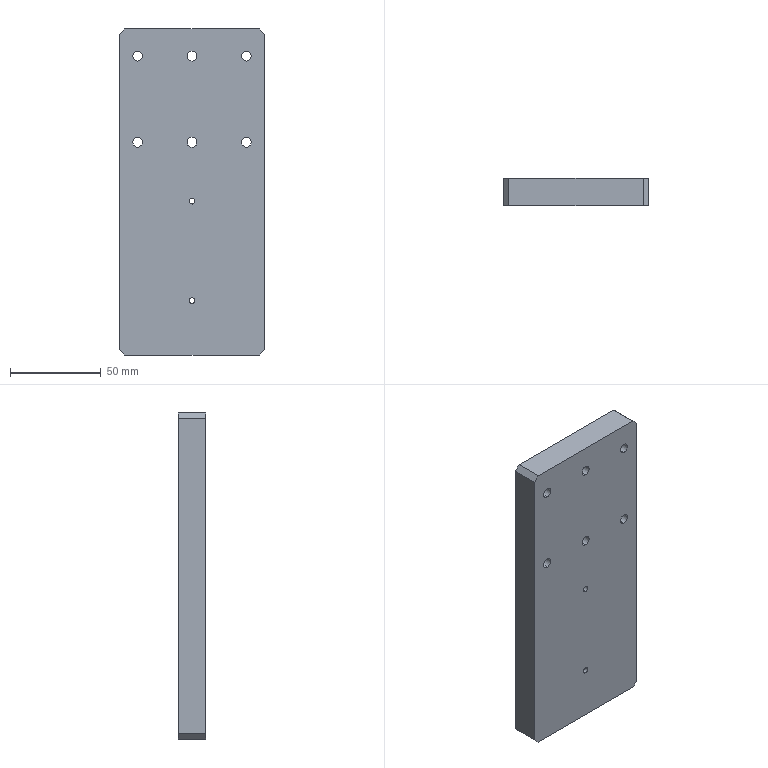Part | SolidWorks | features HoleWzd 3, Chamfer 1, Extrusion 1 | 1 solid | 44 faces | box 80 x 15 x 180 mm | volume 211462 mm3 | cylinder 28 | plane 16 | commonest cylinder face diameters 5.5 x12 10 x12 3.3 x4
STEP:
#1=CARTESIAN_POINT('',(-30.,9.3,70.));
#2=VERTEX_POINT('',#1);
#3=CARTESIAN_POINT('',(-30.,9.3,80.));
#4=VERTEX_POINT('',#3);
#5=CARTESIAN_POINT('',(-30.,9.3,75.));
#6=DIRECTION('',(0.,1.,0.));
#7=DIRECTION('',(0.,0.,1.));
#8=AXIS2_PLACEMENT_3D('',#5,#6,#7);
#9=CIRCLE('',#8,5.);
#10=EDGE_CURVE('',#2,#4,#9,.T.);
#11=ORIENTED_EDGE('',*,*,#10,.F.);
#12=CARTESIAN_POINT('',(-30.,15.,70.));
#13=VERTEX_POINT('',#12);
#14=CARTESIAN_POINT('',(-30.,15.,70.));
#15=DIRECTION('',(0.,1.,0.));
#16=VECTOR('',#15,1000.);
#17=LINE('',#14,#16);
#18=EDGE_CURVE('',#2,#13,#17,.T.);
#19=ORIENTED_EDGE('',*,*,#18,.T.);
#20=CARTESIAN_POINT('',(-30.,15.,80.));
#21=VERTEX_POINT('',#20);
#22=CARTESIAN_POINT('',(-30.,15.,75.));
#23=DIRECTION('',(0.,1.,0.));
#24=DIRECTION('',(0.,0.,1.));
#25=AXIS2_PLACEMENT_3D('',#22,#23,#24);
#26=CIRCLE('',#25,5.);
#27=EDGE_CURVE('',#13,#21,#26,.T.);
#28=ORIENTED_EDGE('',*,*,#27,.T.);
#29=CARTESIAN_POINT('',(-30.,15.,80.));
#30=DIRECTION('',(0.,1.,0.));
#31=VECTOR('',#30,1000.);
#32=LINE('',#29,#31);
#33=EDGE_CURVE('',#4,#21,#32,.T.);
#34=ORIENTED_EDGE('',*,*,#33,.F.);
#35=EDGE_LOOP('',(#11,#19,#28,#34));
#36=FACE_OUTER_BOUND('',#35,.T.);
#37=CARTESIAN_POINT('',(-30.,15.,75.));
#38=DIRECTION('',(0.,1.,0.));
#39=DIRECTION('',(0.,0.,1.));
#40=AXIS2_PLACEMENT_3D('',#37,#38,#39);
#41=CYLINDRICAL_SURFACE('',#40,5.);
#42=ADVANCED_FACE('',(#36),#41,.F.);
#43=CARTESIAN_POINT('',(-30.,0.,72.25));
#44=VERTEX_POINT('',#43);
#45=CARTESIAN_POINT('',(-30.,0.,77.75));
#46=VERTEX_POINT('',#45);
#47=CARTESIAN_POINT('',(-30.,0.,75.));
#48=DIRECTION('',(0.,1.,0.));
#49=DIRECTION('',(0.,0.,1.));
#50=AXIS2_PLACEMENT_3D('',#47,#48,#49);
#51=CIRCLE('',#50,2.75);
#52=EDGE_CURVE('',#44,#46,#51,.T.);
#53=ORIENTED_EDGE('',*,*,#52,.F.);
#54=CARTESIAN_POINT('',(-30.,9.3,72.25));
#55=VERTEX_POINT('',#54);
#56=CARTESIAN_POINT('',(-30.,15.,72.25));
#57=DIRECTION('',(0.,1.,0.));
#58=VECTOR('',#57,1000.);
#59=LINE('',#56,#58);
#60=EDGE_CURVE('',#44,#55,#59,.T.);
#61=ORIENTED_EDGE('',*,*,#60,.T.);
#62=CARTESIAN_POINT('',(-30.,9.3,77.75));
#63=VERTEX_POINT('',#62);
#64=CARTESIAN_POINT('',(-30.,9.3,75.));
#65=DIRECTION('',(0.,1.,0.));
#66=DIRECTION('',(0.,0.,1.));
#67=AXIS2_PLACEMENT_3D('',#64,#65,#66);
#68=CIRCLE('',#67,2.75);
#69=EDGE_CURVE('',#55,#63,#68,.T.);
#70=ORIENTED_EDGE('',*,*,#69,.T.);
#71=CARTESIAN_POINT('',(-30.,15.,77.75));
#72=DIRECTION('',(0.,1.,0.));
#73=VECTOR('',#72,1000.);
#74=LINE('',#71,#73);
#75=EDGE_CURVE('',#46,#63,#74,.T.);
#76=ORIENTED_EDGE('',*,*,#75,.F.);
#77=EDGE_LOOP('',(#53,#61,#70,#76));
#78=FACE_OUTER_BOUND('',#77,.T.);
#79=CARTESIAN_POINT('',(-30.,15.,75.));
#80=DIRECTION('',(0.,1.,0.));
#81=DIRECTION('',(0.,0.,1.));
#82=AXIS2_PLACEMENT_3D('',#79,#80,#81);
#83=CYLINDRICAL_SURFACE('',#82,2.75);
#84=ADVANCED_FACE('',(#78),#83,.F.);
#85=CARTESIAN_POINT('',(0.,9.3,70.));
#86=VERTEX_POINT('',#85);
#87=CARTESIAN_POINT('',(0.,9.3,80.));
#88=VERTEX_POINT('',#87);
#89=CARTESIAN_POINT('',(0.,9.3,75.));
#90=DIRECTION('',(0.,1.,0.));
#91=DIRECTION('',(0.,0.,1.));
#92=AXIS2_PLACEMENT_3D('',#89,#90,#91);
#93=CIRCLE('',#92,5.);
#94=EDGE_CURVE('',#86,#88,#93,.T.);
#95=ORIENTED_EDGE('',*,*,#94,.F.);
#96=CARTESIAN_POINT('',(0.,15.,70.));
#97=VERTEX_POINT('',#96);
#98=CARTESIAN_POINT('',(0.,15.,70.));
#99=DIRECTION('',(0.,1.,0.));
#100=VECTOR('',#99,1000.);
#101=LINE('',#98,#100);
#102=EDGE_CURVE('',#86,#97,#101,.T.);
#103=ORIENTED_EDGE('',*,*,#102,.T.);
#104=CARTESIAN_POINT('',(0.,15.,80.));
#105=VERTEX_POINT('',#104);
#106=CARTESIAN_POINT('',(0.,15.,75.));
#107=DIRECTION('',(0.,1.,0.));
#108=DIRECTION('',(0.,0.,1.));
#109=AXIS2_PLACEMENT_3D('',#106,#107,#108);
#110=CIRCLE('',#109,5.);
#111=EDGE_CURVE('',#97,#105,#110,.T.);
#112=ORIENTED_EDGE('',*,*,#111,.T.);
#113=CARTESIAN_POINT('',(0.,15.,80.));
#114=DIRECTION('',(0.,1.,0.));
#115=VECTOR('',#114,1000.);
#116=LINE('',#113,#115);
#117=EDGE_CURVE('',#88,#105,#116,.T.);
#118=ORIENTED_EDGE('',*,*,#117,.F.);
#119=EDGE_LOOP('',(#95,#103,#112,#118));
#120=FACE_OUTER_BOUND('',#119,.T.);
#121=CARTESIAN_POINT('',(0.,15.,75.));
#122=DIRECTION('',(0.,1.,0.));
#123=DIRECTION('',(0.,0.,1.));
#124=AXIS2_PLACEMENT_3D('',#121,#122,#123);
#125=CYLINDRICAL_SURFACE('',#124,5.);
#126=ADVANCED_FACE('',(#120),#125,.F.);
#127=CARTESIAN_POINT('',(0.,0.,72.25));
#128=VERTEX_POINT('',#127);
#129=CARTESIAN_POINT('',(0.,0.,77.75));
#130=VERTEX_POINT('',#129);
#131=CARTESIAN_POINT('',(0.,0.,75.));
#132=DIRECTION('',(0.,1.,0.));
#133=DIRECTION('',(0.,0.,1.));
#134=AXIS2_PLACEMENT_3D('',#131,#132,#133);
#135=CIRCLE('',#134,2.75);
#136=EDGE_CURVE('',#128,#130,#135,.T.);
#137=ORIENTED_EDGE('',*,*,#136,.F.);
#138=CARTESIAN_POINT('',(0.,9.3,72.25));
#139=VERTEX_POINT('',#138);
#140=CARTESIAN_POINT('',(0.,15.,72.25));
#141=DIRECTION('',(0.,1.,0.));
#142=VECTOR('',#141,1000.);
#143=LINE('',#140,#142);
#144=EDGE_CURVE('',#128,#139,#143,.T.);
#145=ORIENTED_EDGE('',*,*,#144,.T.);
#146=CARTESIAN_POINT('',(0.,9.3,77.75));
#147=VERTEX_POINT('',#146);
#148=CARTESIAN_POINT('',(0.,9.3,75.));
#149=DIRECTION('',(0.,1.,0.));
#150=DIRECTION('',(0.,0.,1.));
#151=AXIS2_PLACEMENT_3D('',#148,#149,#150);
#152=CIRCLE('',#151,2.75);
#153=EDGE_CURVE('',#139,#147,#152,.T.);
#154=ORIENTED_EDGE('',*,*,#153,.T.);
#155=CARTESIAN_POINT('',(0.,15.,77.75));
#156=DIRECTION('',(0.,1.,0.));
#157=VECTOR('',#156,1000.);
#158=LINE('',#155,#157);
#159=EDGE_CURVE('',#130,#147,#158,.T.);
#160=ORIENTED_EDGE('',*,*,#159,.F.);
#161=EDGE_LOOP('',(#137,#145,#154,#160));
#162=FACE_OUTER_BOUND('',#161,.T.);
#163=CARTESIAN_POINT('',(0.,15.,75.));
#164=DIRECTION('',(0.,1.,0.));
#165=DIRECTION('',(0.,0.,1.));
#166=AXIS2_PLACEMENT_3D('',#163,#164,#165);
#167=CYLINDRICAL_SURFACE('',#166,2.75);
#168=ADVANCED_FACE('',(#162),#167,.F.);
#169=CARTESIAN_POINT('',(30.,9.3,70.));
#170=VERTEX_POINT('',#169);
#171=CARTESIAN_POINT('',(30.,9.3,80.));
#172=VERTEX_POINT('',#171);
#173=CARTESIAN_POINT('',(30.,9.3,75.));
#174=DIRECTION('',(0.,1.,0.));
#175=DIRECTION('',(0.,0.,1.));
#176=AXIS2_PLACEMENT_3D('',#173,#174,#175);
#177=CIRCLE('',#176,5.);
#178=EDGE_CURVE('',#170,#172,#177,.T.);
#179=ORIENTED_EDGE('',*,*,#178,.F.);
#180=CARTESIAN_POINT('',(30.,15.,70.));
#181=VERTEX_POINT('',#180);
#182=CARTESIAN_POINT('',(30.,15.,70.));
#183=DIRECTION('',(0.,1.,0.));
#184=VECTOR('',#183,1000.);
#185=LINE('',#182,#184);
#186=EDGE_CURVE('',#170,#181,#185,.T.);
#187=ORIENTED_EDGE('',*,*,#186,.T.);
#188=CARTESIAN_POINT('',(30.,15.,80.));
#189=VERTEX_POINT('',#188);
#190=CARTESIAN_POINT('',(30.,15.,75.));
#191=DIRECTION('',(0.,1.,0.));
#192=DIRECTION('',(0.,0.,1.));
#193=AXIS2_PLACEMENT_3D('',#190,#191,#192);
#194=CIRCLE('',#193,5.);
#195=EDGE_CURVE('',#181,#189,#194,.T.);
#196=ORIENTED_EDGE('',*,*,#195,.T.);
#197=CARTESIAN_POINT('',(30.,15.,80.));
#198=DIRECTION('',(0.,1.,0.));
#199=VECTOR('',#198,1000.);
#200=LINE('',#197,#199);
#201=EDGE_CURVE('',#172,#189,#200,.T.);
#202=ORIENTED_EDGE('',*,*,#201,.F.);
#203=EDGE_LOOP('',(#179,#187,#196,#202));
#204=FACE_OUTER_BOUND('',#203,.T.);
#205=CARTESIAN_POINT('',(30.,15.,75.));
#206=DIRECTION('',(0.,1.,0.));
#207=DIRECTION('',(0.,0.,1.));
#208=AXIS2_PLACEMENT_3D('',#205,#206,#207);
#209=CYLINDRICAL_SURFACE('',#208,5.);
#210=ADVANCED_FACE('',(#204),#209,.F.);
#211=CARTESIAN_POINT('',(30.,0.,72.25));
#212=VERTEX_POINT('',#211);
#213=CARTESIAN_POINT('',(30.,0.,77.75));
#214=VERTEX_POINT('',#213);
#215=CARTESIAN_POINT('',(30.,0.,75.));
#216=DIRECTION('',(0.,1.,0.));
#217=DIRECTION('',(0.,0.,1.));
#218=AXIS2_PLACEMENT_3D('',#215,#216,#217);
#219=CIRCLE('',#218,2.75);
#220=EDGE_CURVE('',#212,#214,#219,.T.);
#221=ORIENTED_EDGE('',*,*,#220,.F.);
#222=CARTESIAN_POINT('',(30.,9.3,72.25));
#223=VERTEX_POINT('',#222);
#224=CARTESIAN_POINT('',(30.,15.,72.25));
#225=DIRECTION('',(0.,1.,0.));
#226=VECTOR('',#225,1000.);
#227=LINE('',#224,#226);
#228=EDGE_CURVE('',#212,#223,#227,.T.);
#229=ORIENTED_EDGE('',*,*,#228,.T.);
#230=CARTESIAN_POINT('',(30.,9.3,77.75));
#231=VERTEX_POINT('',#230);
#232=CARTESIAN_POINT('',(30.,9.3,75.));
#233=DIRECTION('',(0.,1.,0.));
#234=DIRECTION('',(0.,0.,1.));
#235=AXIS2_PLACEMENT_3D('',#232,#233,#234);
#236=CIRCLE('',#235,2.75);
#237=EDGE_CURVE('',#223,#231,#236,.T.);
#238=ORIENTED_EDGE('',*,*,#237,.T.);
#239=CARTESIAN_POINT('',(30.,15.,77.75));
#240=DIRECTION('',(0.,1.,0.));
#241=VECTOR('',#240,1000.);
#242=LINE('',#239,#241);
#243=EDGE_CURVE('',#214,#231,#242,.T.);
#244=ORIENTED_EDGE('',*,*,#243,.F.);
#245=EDGE_LOOP('',(#221,#229,#238,#244));
#246=FACE_OUTER_BOUND('',#245,.T.);
#247=CARTESIAN_POINT('',(30.,15.,75.));
#248=DIRECTION('',(0.,1.,0.));
#249=DIRECTION('',(0.,0.,1.));
#250=AXIS2_PLACEMENT_3D('',#247,#248,#249);
#251=CYLINDRICAL_SURFACE('',#250,2.75);
#252=ADVANCED_FACE('',(#246),#251,.F.);
#253=CARTESIAN_POINT('',(-30.,9.3,22.5));
#254=VERTEX_POINT('',#253);
#255=CARTESIAN_POINT('',(-30.,9.3,32.5));
#256=VERTEX_POINT('',#255);
#257=CARTESIAN_POINT('',(-30.,9.3,27.5));
#258=DIRECTION('',(0.,1.,0.));
#259=DIRECTION('',(0.,0.,1.));
#260=AXIS2_PLACEMENT_3D('',#257,#258,#259);
#261=CIRCLE('',#260,5.);
#262=EDGE_CURVE('',#254,#256,#261,.T.);
#263=ORIENTED_EDGE('',*,*,#262,.F.);
#264=CARTESIAN_POINT('',(-30.,15.,22.5));
#265=VERTEX_POINT('',#264);
#266=CARTESIAN_POINT('',(-30.,15.,22.5));
#267=DIRECTION('',(0.,1.,0.));
#268=VECTOR('',#267,1000.);
#269=LINE('',#266,#268);
#270=EDGE_CURVE('',#254,#265,#269,.T.);
#271=ORIENTED_EDGE('',*,*,#270,.T.);
#272=CARTESIAN_POINT('',(-30.,15.,32.5));
#273=VERTEX_POINT('',#272);
#274=CARTESIAN_POINT('',(-30.,15.,27.5));
#275=DIRECTION('',(0.,1.,0.));
#276=DIRECTION('',(0.,0.,1.));
#277=AXIS2_PLACEMENT_3D('',#274,#275,#276);
#278=CIRCLE('',#277,5.);
#279=EDGE_CURVE('',#265,#273,#278,.T.);
#280=ORIENTED_EDGE('',*,*,#279,.T.);
#281=CARTESIAN_POINT('',(-30.,15.,32.5));
#282=DIRECTION('',(0.,1.,0.));
#283=VECTOR('',#282,1000.);
#284=LINE('',#281,#283);
#285=EDGE_CURVE('',#256,#273,#284,.T.);
#286=ORIENTED_EDGE('',*,*,#285,.F.);
#287=EDGE_LOOP('',(#263,#271,#280,#286));
#288=FACE_OUTER_BOUND('',#287,.T.);
#289=CARTESIAN_POINT('',(-30.,15.,27.5));
#290=DIRECTION('',(0.,1.,0.));
#291=DIRECTION('',(0.,0.,1.));
#292=AXIS2_PLACEMENT_3D('',#289,#290,#291);
#293=CYLINDRICAL_SURFACE('',#292,5.);
#294=ADVANCED_FACE('',(#288),#293,.F.);
#295=CARTESIAN_POINT('',(-30.,0.,24.75));
#296=VERTEX_POINT('',#295);
#297=CARTESIAN_POINT('',(-30.,0.,30.25));
#298=VERTEX_POINT('',#297);
#299=CARTESIAN_POINT('',(-30.,0.,27.5));
#300=DIRECTION('',(0.,1.,0.));
#301=DIRECTION('',(0.,0.,1.));
#302=AXIS2_PLACEMENT_3D('',#299,#300,#301);
#303=CIRCLE('',#302,2.75);
#304=EDGE_CURVE('',#296,#298,#303,.T.);
#305=ORIENTED_EDGE('',*,*,#304,.F.);
#306=CARTESIAN_POINT('',(-30.,9.3,24.75));
#307=VERTEX_POINT('',#306);
#308=CARTESIAN_POINT('',(-30.,15.,24.75));
#309=DIRECTION('',(0.,1.,0.));
#310=VECTOR('',#309,1000.);
#311=LINE('',#308,#310);
#312=EDGE_CURVE('',#296,#307,#311,.T.);
#313=ORIENTED_EDGE('',*,*,#312,.T.);
#314=CARTESIAN_POINT('',(-30.,9.3,30.25));
#315=VERTEX_POINT('',#314);
#316=CARTESIAN_POINT('',(-30.,9.3,27.5));
#317=DIRECTION('',(0.,1.,0.));
#318=DIRECTION('',(0.,0.,1.));
#319=AXIS2_PLACEMENT_3D('',#316,#317,#318);
#320=CIRCLE('',#319,2.75);
#321=EDGE_CURVE('',#307,#315,#320,.T.);
#322=ORIENTED_EDGE('',*,*,#321,.T.);
#323=CARTESIAN_POINT('',(-30.,15.,30.25));
#324=DIRECTION('',(0.,1.,0.));
#325=VECTOR('',#324,1000.);
#326=LINE('',#323,#325);
#327=EDGE_CURVE('',#298,#315,#326,.T.);
#328=ORIENTED_EDGE('',*,*,#327,.F.);
#329=EDGE_LOOP('',(#305,#313,#322,#328));
#330=FACE_OUTER_BOUND('',#329,.T.);
#331=CARTESIAN_POINT('',(-30.,15.,27.5));
#332=DIRECTION('',(0.,1.,0.));
#333=DIRECTION('',(0.,0.,1.));
#334=AXIS2_PLACEMENT_3D('',#331,#332,#333);
#335=CYLINDRICAL_SURFACE('',#334,2.75);
#336=ADVANCED_FACE('',(#330),#335,.F.);
#337=CARTESIAN_POINT('',(0.,9.3,22.5));
#338=VERTEX_POINT('',#337);
#339=CARTESIAN_POINT('',(0.,9.3,32.5));
#340=VERTEX_POINT('',#339);
#341=CARTESIAN_POINT('',(0.,9.3,27.5));
#342=DIRECTION('',(0.,1.,0.));
#343=DIRECTION('',(0.,0.,1.));
#344=AXIS2_PLACEMENT_3D('',#341,#342,#343);
#345=CIRCLE('',#344,5.);
#346=EDGE_CURVE('',#338,#340,#345,.T.);
#347=ORIENTED_EDGE('',*,*,#346,.F.);
#348=CARTESIAN_POINT('',(0.,15.,22.5));
#349=VERTEX_POINT('',#348);
#350=CARTESIAN_POINT('',(0.,15.,22.5));
#351=DIRECTION('',(0.,1.,0.));
#352=VECTOR('',#351,1000.);
#353=LINE('',#350,#352);
#354=EDGE_CURVE('',#338,#349,#353,.T.);
#355=ORIENTED_EDGE('',*,*,#354,.T.);
#356=CARTESIAN_POINT('',(0.,15.,32.5));
#357=VERTEX_POINT('',#356);
#358=CARTESIAN_POINT('',(0.,15.,27.5));
#359=DIRECTION('',(0.,1.,0.));
#360=DIRECTION('',(0.,0.,1.));
#361=AXIS2_PLACEMENT_3D('',#358,#359,#360);
#362=CIRCLE('',#361,5.);
#363=EDGE_CURVE('',#349,#357,#362,.T.);
#364=ORIENTED_EDGE('',*,*,#363,.T.);
#365=CARTESIAN_POINT('',(0.,15.,32.5));
#366=DIRECTION('',(0.,1.,0.));
#367=VECTOR('',#366,1000.);
#368=LINE('',#365,#367);
#369=EDGE_CURVE('',#340,#357,#368,.T.);
#370=ORIENTED_EDGE('',*,*,#369,.F.);
#371=EDGE_LOOP('',(#347,#355,#364,#370));
#372=FACE_OUTER_BOUND('',#371,.T.);
#373=CARTESIAN_POINT('',(0.,15.,27.5));
#374=DIRECTION('',(0.,1.,0.));
#375=DIRECTION('',(0.,0.,1.));
#376=AXIS2_PLACEMENT_3D('',#373,#374,#375);
#377=CYLINDRICAL_SURFACE('',#376,5.);
#378=ADVANCED_FACE('',(#372),#377,.F.);
#379=CARTESIAN_POINT('',(0.,0.,24.75));
#380=VERTEX_POINT('',#379);
#381=CARTESIAN_POINT('',(0.,0.,30.25));
#382=VERTEX_POINT('',#381);
#383=CARTESIAN_POINT('',(0.,0.,27.5));
#384=DIRECTION('',(0.,1.,0.));
#385=DIRECTION('',(0.,0.,1.));
#386=AXIS2_PLACEMENT_3D('',#383,#384,#385);
#387=CIRCLE('',#386,2.75);
#388=EDGE_CURVE('',#380,#382,#387,.T.);
#389=ORIENTED_EDGE('',*,*,#388,.F.);
#390=CARTESIAN_POINT('',(0.,9.3,24.75));
#391=VERTEX_POINT('',#390);
#392=CARTESIAN_POINT('',(0.,15.,24.75));
#393=DIRECTION('',(0.,1.,0.));
#394=VECTOR('',#393,1000.);
#395=LINE('',#392,#394);
#396=EDGE_CURVE('',#380,#391,#395,.T.);
#397=ORIENTED_EDGE('',*,*,#396,.T.);
#398=CARTESIAN_POINT('',(0.,9.3,30.25));
#399=VERTEX_POINT('',#398);
#400=CARTESIAN_POINT('',(0.,9.3,27.5));
#401=DIRECTION('',(0.,1.,0.));
#402=DIRECTION('',(0.,0.,1.));
#403=AXIS2_PLACEMENT_3D('',#400,#401,#402);
#404=CIRCLE('',#403,2.75);
#405=EDGE_CURVE('',#391,#399,#404,.T.);
#406=ORIENTED_EDGE('',*,*,#405,.T.);
#407=CARTESIAN_POINT('',(0.,15.,30.25));
#408=DIRECTION('',(0.,1.,0.));
#409=VECTOR('',#408,1000.);
#410=LINE('',#407,#409);
#411=EDGE_CURVE('',#382,#399,#410,.T.);
#412=ORIENTED_EDGE('',*,*,#411,.F.);
#413=EDGE_LOOP('',(#389,#397,#406,#412));
#414=FACE_OUTER_BOUND('',#413,.T.);
#415=CARTESIAN_POINT('',(0.,15.,27.5));
#416=DIRECTION('',(0.,1.,0.));
#417=DIRECTION('',(0.,0.,1.));
#418=AXIS2_PLACEMENT_3D('',#415,#416,#417);
#419=CYLINDRICAL_SURFACE('',#418,2.75);
#420=ADVANCED_FACE('',(#414),#419,.F.);
#421=CARTESIAN_POINT('',(30.,9.3,22.5));
#422=VERTEX_POINT('',#421);
#423=CARTESIAN_POINT('',(30.,9.3,32.5));
#424=VERTEX_POINT('',#423);
#425=CARTESIAN_POINT('',(30.,9.3,27.5));
#426=DIRECTION('',(0.,1.,0.));
#427=DIRECTION('',(0.,0.,1.));
#428=AXIS2_PLACEMENT_3D('',#425,#426,#427);
#429=CIRCLE('',#428,5.);
#430=EDGE_CURVE('',#422,#424,#429,.T.);
#431=ORIENTED_EDGE('',*,*,#430,.F.);
#432=CARTESIAN_POINT('',(30.,15.,22.5));
#433=VERTEX_POINT('',#432);
#434=CARTESIAN_POINT('',(30.,15.,22.5));
#435=DIRECTION('',(0.,1.,0.));
#436=VECTOR('',#435,1000.);
#437=LINE('',#434,#436);
#438=EDGE_CURVE('',#422,#433,#437,.T.);
#439=ORIENTED_EDGE('',*,*,#438,.T.);
#440=CARTESIAN_POINT('',(30.,15.,32.5));
#441=VERTEX_POINT('',#440);
#442=CARTESIAN_POINT('',(30.,15.,27.5));
#443=DIRECTION('',(0.,1.,0.));
#444=DIRECTION('',(0.,0.,1.));
#445=AXIS2_PLACEMENT_3D('',#442,#443,#444);
#446=CIRCLE('',#445,5.);
#447=EDGE_CURVE('',#433,#441,#446,.T.);
#448=ORIENTED_EDGE('',*,*,#447,.T.);
#449=CARTESIAN_POINT('',(30.,15.,32.5));
#450=DIRECTION('',(0.,1.,0.));
#451=VECTOR('',#450,1000.);
#452=LINE('',#449,#451);
#453=EDGE_CURVE('',#424,#441,#452,.T.);
#454=ORIENTED_EDGE('',*,*,#453,.F.);
#455=EDGE_LOOP('',(#431,#439,#448,#454));
#456=FACE_OUTER_BOUND('',#455,.T.);
#457=CARTESIAN_POINT('',(30.,15.,27.5));
#458=DIRECTION('',(0.,1.,0.));
#459=DIRECTION('',(0.,0.,1.));
#460=AXIS2_PLACEMENT_3D('',#457,#458,#459);
#461=CYLINDRICAL_SURFACE('',#460,5.);
#462=ADVANCED_FACE('',(#456),#461,.F.);
#463=CARTESIAN_POINT('',(30.,0.,24.75));
#464=VERTEX_POINT('',#463);
#465=CARTESIAN_POINT('',(30.,0.,30.25));
#466=VERTEX_POINT('',#465);
#467=CARTESIAN_POINT('',(30.,0.,27.5));
#468=DIRECTION('',(0.,1.,0.));
#469=DIRECTION('',(0.,0.,1.));
#470=AXIS2_PLACEMENT_3D('',#467,#468,#469);
#471=CIRCLE('',#470,2.75);
#472=EDGE_CURVE('',#464,#466,#471,.T.);
#473=ORIENTED_EDGE('',*,*,#472,.F.);
#474=CARTESIAN_POINT('',(30.,9.3,24.75));
#475=VERTEX_POINT('',#474);
#476=CARTESIAN_POINT('',(30.,15.,24.75));
#477=DIRECTION('',(0.,1.,0.));
#478=VECTOR('',#477,1000.);
#479=LINE('',#476,#478);
#480=EDGE_CURVE('',#464,#475,#479,.T.);
#481=ORIENTED_EDGE('',*,*,#480,.T.);
#482=CARTESIAN_POINT('',(30.,9.3,30.25));
#483=VERTEX_POINT('',#482);
#484=CARTESIAN_POINT('',(30.,9.3,27.5));
#485=DIRECTION('',(0.,1.,0.));
#486=DIRECTION('',(0.,0.,1.));
#487=AXIS2_PLACEMENT_3D('',#484,#485,#486);
#488=CIRCLE('',#487,2.75);
#489=EDGE_CURVE('',#475,#483,#488,.T.);
#490=ORIENTED_EDGE('',*,*,#489,.T.);
#491=CARTESIAN_POINT('',(30.,15.,30.25));
#492=DIRECTION('',(0.,1.,0.));
#493=VECTOR('',#492,1000.);
#494=LINE('',#491,#493);
#495=EDGE_CURVE('',#466,#483,#494,.T.);
#496=ORIENTED_EDGE('',*,*,#495,.F.);
#497=EDGE_LOOP('',(#473,#481,#490,#496));
#498=FACE_OUTER_BOUND('',#497,.T.);
#499=CARTESIAN_POINT('',(30.,15.,27.5));
#500=DIRECTION('',(0.,1.,0.));
#501=DIRECTION('',(0.,0.,1.));
#502=AXIS2_PLACEMENT_3D('',#499,#500,#501);
#503=CYLINDRICAL_SURFACE('',#502,2.75);
#504=ADVANCED_FACE('',(#498),#503,.F.);
#505=CARTESIAN_POINT('',(0.,0.,-61.65));
#506=VERTEX_POINT('',#505);
#507=CARTESIAN_POINT('',(0.,0.,-58.35));
#508=VERTEX_POINT('',#507);
#509=CARTESIAN_POINT('',(0.,0.,-60.));
#510=DIRECTION('',(0.,1.,0.));
#511=DIRECTION('',(0.,0.,1.));
#512=AXIS2_PLACEMENT_3D('',#509,#510,#511);
#513=CIRCLE('',#512,1.65);
#514=EDGE_CURVE('',#506,#508,#513,.T.);
#515=ORIENTED_EDGE('',*,*,#514,.F.);
#516=CARTESIAN_POINT('',(0.,15.,-61.65));
#517=VERTEX_POINT('',#516);
#518=CARTESIAN_POINT('',(0.,15.,-61.65));
#519=DIRECTION('',(0.,1.,0.));
#520=VECTOR('',#519,1000.);
#521=LINE('',#518,#520);
#522=EDGE_CURVE('',#506,#517,#521,.T.);
#523=ORIENTED_EDGE('',*,*,#522,.T.);
#524=CARTESIAN_POINT('',(0.,15.,-58.35));
#525=VERTEX_POINT('',#524);
#526=CARTESIAN_POINT('',(0.,15.,-60.));
#527=DIRECTION('',(0.,1.,0.));
#528=DIRECTION('',(0.,0.,1.));
#529=AXIS2_PLACEMENT_3D('',#526,#527,#528);
#530=CIRCLE('',#529,1.65);
#531=EDGE_CURVE('',#517,#525,#530,.T.);
#532=ORIENTED_EDGE('',*,*,#531,.T.);
#533=CARTESIAN_POINT('',(0.,15.,-58.35));
#534=DIRECTION('',(0.,1.,0.));
#535=VECTOR('',#534,1000.);
#536=LINE('',#533,#535);
#537=EDGE_CURVE('',#508,#525,#536,.T.);
#538=ORIENTED_EDGE('',*,*,#537,.F.);
#539=EDGE_LOOP('',(#515,#523,#532,#538));
#540=FACE_OUTER_BOUND('',#539,.T.);
#541=CARTESIAN_POINT('',(0.,15.,-60.));
#542=DIRECTION('',(0.,1.,0.));
#543=DIRECTION('',(0.,0.,1.));
#544=AXIS2_PLACEMENT_3D('',#541,#542,#543);
#545=CYLINDRICAL_SURFACE('',#544,1.65);
#546=ADVANCED_FACE('',(#540),#545,.F.);
#547=CARTESIAN_POINT('',(0.,0.,-6.65));
#548=VERTEX_POINT('',#547);
#549=CARTESIAN_POINT('',(0.,0.,-3.35));
#550=VERTEX_POINT('',#549);
#551=CARTESIAN_POINT('',(0.,0.,-5.));
#552=DIRECTION('',(0.,1.,0.));
#553=DIRECTION('',(0.,0.,1.));
#554=AXIS2_PLACEMENT_3D('',#551,#552,#553);
#555=CIRCLE('',#554,1.65);
#556=EDGE_CURVE('',#548,#550,#555,.T.);
#557=ORIENTED_EDGE('',*,*,#556,.F.);
#558=CARTESIAN_POINT('',(0.,15.,-6.65));
#559=VERTEX_POINT('',#558);
#560=CARTESIAN_POINT('',(0.,15.,-6.65));
#561=DIRECTION('',(0.,1.,0.));
#562=VECTOR('',#561,1000.);
#563=LINE('',#560,#562);
#564=EDGE_CURVE('',#548,#559,#563,.T.);
#565=ORIENTED_EDGE('',*,*,#564,.T.);
#566=CARTESIAN_POINT('',(0.,15.,-3.35));
#567=VERTEX_POINT('',#566);
#568=CARTESIAN_POINT('',(0.,15.,-5.));
#569=DIRECTION('',(0.,1.,0.));
#570=DIRECTION('',(0.,0.,1.));
#571=AXIS2_PLACEMENT_3D('',#568,#569,#570);
#572=CIRCLE('',#571,1.65);
#573=EDGE_CURVE('',#559,#567,#572,.T.);
#574=ORIENTED_EDGE('',*,*,#573,.T.);
#575=CARTESIAN_POINT('',(0.,15.,-3.35));
#576=DIRECTION('',(0.,1.,0.));
#577=VECTOR('',#576,1000.);
#578=LINE('',#575,#577);
#579=EDGE_CURVE('',#550,#567,#578,.T.);
#580=ORIENTED_EDGE('',*,*,#579,.F.);
#581=EDGE_LOOP('',(#557,#565,#574,#580));
#582=FACE_OUTER_BOUND('',#581,.T.);
#583=CARTESIAN_POINT('',(0.,15.,-5.));
#584=DIRECTION('',(0.,1.,0.));
#585=DIRECTION('',(0.,0.,1.));
#586=AXIS2_PLACEMENT_3D('',#583,#584,#585);
#587=CYLINDRICAL_SURFACE('',#586,1.65);
#588=ADVANCED_FACE('',(#582),#587,.F.);
#589=CARTESIAN_POINT('',(40.,0.,87.));
#590=VERTEX_POINT('',#589);
#591=CARTESIAN_POINT('',(40.,0.,-87.));
#592=VERTEX_POINT('',#591);
#593=CARTESIAN_POINT('',(40.,0.,-90.));
#594=DIRECTION('',(0.,0.,-1.));
#595=VECTOR('',#594,1000.);
#596=LINE('',#593,#595);
#597=EDGE_CURVE('',#590,#592,#596,.T.);
#598=ORIENTED_EDGE('',*,*,#597,.T.);
#599=CARTESIAN_POINT('',(40.,15.,-87.));
#600=VERTEX_POINT('',#599);
#601=CARTESIAN_POINT('',(40.,15.,-87.));
#602=DIRECTION('',(0.,1.,0.));
#603=VECTOR('',#602,1000.);
#604=LINE('',#601,#603);
#605=EDGE_CURVE('',#592,#600,#604,.T.);
#606=ORIENTED_EDGE('',*,*,#605,.T.);
#607=CARTESIAN_POINT('',(40.,15.,87.));
#608=VERTEX_POINT('',#607);
#609=CARTESIAN_POINT('',(40.,15.,-90.));
#610=DIRECTION('',(0.,0.,-1.));
#611=VECTOR('',#610,1000.);
#612=LINE('',#609,#611);
#613=EDGE_CURVE('',#608,#600,#612,.T.);
#614=ORIENTED_EDGE('',*,*,#613,.F.);
#615=CARTESIAN_POINT('',(40.,15.,87.));
#616=DIRECTION('',(0.,-1.,0.));
#617=VECTOR('',#616,1000.);
#618=LINE('',#615,#617);
#619=EDGE_CURVE('',#608,#590,#618,.T.);
#620=ORIENTED_EDGE('',*,*,#619,.T.);
#621=EDGE_LOOP('',(#598,#606,#614,#620));
#622=FACE_OUTER_BOUND('',#621,.T.);
#623=CARTESIAN_POINT('',(40.,15.,-90.));
#624=DIRECTION('',(-1.,0.,0.));
#625=DIRECTION('',(0.,0.,1.));
#626=AXIS2_PLACEMENT_3D('',#623,#624,#625);
#627=PLANE('',#626);
#628=ADVANCED_FACE('',(#622),#627,.F.);
#629=CARTESIAN_POINT('',(37.,0.,-90.));
#630=VERTEX_POINT('',#629);
#631=CARTESIAN_POINT('',(-37.,0.,-90.));
#632=VERTEX_POINT('',#631);
#633=CARTESIAN_POINT('',(-40.,0.,-90.));
#634=DIRECTION('',(-1.,0.,0.));
#635=VECTOR('',#634,1000.);
#636=LINE('',#633,#635);
#637=EDGE_CURVE('',#630,#632,#636,.T.);
#638=ORIENTED_EDGE('',*,*,#637,.T.);
#639=CARTESIAN_POINT('',(-37.,15.,-90.));
#640=VERTEX_POINT('',#639);
#641=CARTESIAN_POINT('',(-37.,15.,-90.));
#642=DIRECTION('',(0.,1.,0.));
#643=VECTOR('',#642,1000.);
#644=LINE('',#641,#643);
#645=EDGE_CURVE('',#632,#640,#644,.T.);
#646=ORIENTED_EDGE('',*,*,#645,.T.);
#647=CARTESIAN_POINT('',(37.,15.,-90.));
#648=VERTEX_POINT('',#647);
#649=CARTESIAN_POINT('',(-40.,15.,-90.));
#650=DIRECTION('',(-1.,0.,0.));
#651=VECTOR('',#650,1000.);
#652=LINE('',#649,#651);
#653=EDGE_CURVE('',#648,#640,#652,.T.);
#654=ORIENTED_EDGE('',*,*,#653,.F.);
#655=CARTESIAN_POINT('',(37.,15.,-90.));
#656=DIRECTION('',(0.,-1.,0.));
#657=VECTOR('',#656,1000.);
#658=LINE('',#655,#657);
#659=EDGE_CURVE('',#648,#630,#658,.T.);
#660=ORIENTED_EDGE('',*,*,#659,.T.);
#661=EDGE_LOOP('',(#638,#646,#654,#660));
#662=FACE_OUTER_BOUND('',#661,.T.);
#663=CARTESIAN_POINT('',(-40.,15.,-90.));
#664=DIRECTION('',(0.,0.,1.));
#665=DIRECTION('',(1.,0.,0.));
#666=AXIS2_PLACEMENT_3D('',#663,#664,#665);
#667=PLANE('',#666);
#668=ADVANCED_FACE('',(#662),#667,.F.);
#669=CARTESIAN_POINT('',(-40.,15.,-87.));
#670=VERTEX_POINT('',#669);
#671=CARTESIAN_POINT('',(-40.,15.,87.));
#672=VERTEX_POINT('',#671);
#673=CARTESIAN_POINT('',(-40.,15.,-90.));
#674=DIRECTION('',(0.,0.,1.));
#675=VECTOR('',#674,1000.);
#676=LINE('',#673,#675);
#677=EDGE_CURVE('',#670,#672,#676,.T.);
#678=ORIENTED_EDGE('',*,*,#677,.F.);
#679=CARTESIAN_POINT('',(-40.,0.,-87.));
#680=VERTEX_POINT('',#679);
#681=CARTESIAN_POINT('',(-40.,15.,-87.));
#682=DIRECTION('',(0.,-1.,0.));
#683=VECTOR('',#682,1000.);
#684=LINE('',#681,#683);
#685=EDGE_CURVE('',#670,#680,#684,.T.);
#686=ORIENTED_EDGE('',*,*,#685,.T.);
#687=CARTESIAN_POINT('',(-40.,0.,87.));
#688=VERTEX_POINT('',#687);
#689=CARTESIAN_POINT('',(-40.,0.,-90.));
#690=DIRECTION('',(0.,0.,1.));
#691=VECTOR('',#690,1000.);
#692=LINE('',#689,#691);
#693=EDGE_CURVE('',#680,#688,#692,.T.);
#694=ORIENTED_EDGE('',*,*,#693,.T.);
#695=CARTESIAN_POINT('',(-40.,15.,87.));
#696=DIRECTION('',(0.,1.,0.));
#697=VECTOR('',#696,1000.);
#698=LINE('',#695,#697);
#699=EDGE_CURVE('',#688,#672,#698,.T.);
#700=ORIENTED_EDGE('',*,*,#699,.T.);
#701=EDGE_LOOP('',(#678,#686,#694,#700));
#702=FACE_OUTER_BOUND('',#701,.T.);
#703=CARTESIAN_POINT('',(-40.,15.,-90.));
#704=DIRECTION('',(1.,0.,0.));
#705=DIRECTION('',(0.,0.,-1.));
#706=AXIS2_PLACEMENT_3D('',#703,#704,#705);
#707=PLANE('',#706);
#708=ADVANCED_FACE('',(#702),#707,.F.);
#709=CARTESIAN_POINT('',(-37.,0.,90.));
#710=VERTEX_POINT('',#709);
#711=CARTESIAN_POINT('',(37.,0.,90.));
#712=VERTEX_POINT('',#711);
#713=CARTESIAN_POINT('',(-40.,0.,90.));
#714=DIRECTION('',(1.,0.,0.));
#715=VECTOR('',#714,1000.);
#716=LINE('',#713,#715);
#717=EDGE_CURVE('',#710,#712,#716,.T.);
#718=ORIENTED_EDGE('',*,*,#717,.T.);
#719=CARTESIAN_POINT('',(37.,15.,90.));
#720=VERTEX_POINT('',#719);
#721=CARTESIAN_POINT('',(37.,15.,90.));
#722=DIRECTION('',(0.,1.,0.));
#723=VECTOR('',#722,1000.);
#724=LINE('',#721,#723);
#725=EDGE_CURVE('',#712,#720,#724,.T.);
#726=ORIENTED_EDGE('',*,*,#725,.T.);
#727=CARTESIAN_POINT('',(-37.,15.,90.));
#728=VERTEX_POINT('',#727);
#729=CARTESIAN_POINT('',(-40.,15.,90.));
#730=DIRECTION('',(1.,0.,0.));
#731=VECTOR('',#730,1000.);
#732=LINE('',#729,#731);
#733=EDGE_CURVE('',#728,#720,#732,.T.);
#734=ORIENTED_EDGE('',*,*,#733,.F.);
#735=CARTESIAN_POINT('',(-37.,15.,90.));
#736=DIRECTION('',(0.,-1.,0.));
#737=VECTOR('',#736,1000.);
#738=LINE('',#735,#737);
#739=EDGE_CURVE('',#728,#710,#738,.T.);
#740=ORIENTED_EDGE('',*,*,#739,.T.);
#741=EDGE_LOOP('',(#718,#726,#734,#740));
#742=FACE_OUTER_BOUND('',#741,.T.);
#743=CARTESIAN_POINT('',(-40.,15.,90.));
#744=DIRECTION('',(0.,0.,-1.));
#745=DIRECTION('',(-1.,0.,0.));
#746=AXIS2_PLACEMENT_3D('',#743,#744,#745);
#747=PLANE('',#746);
#748=ADVANCED_FACE('',(#742),#747,.F.);
#749=CARTESIAN_POINT('',(-30.,15.,75.));
#750=DIRECTION('',(0.,1.,0.));
#751=DIRECTION('',(0.,0.,1.));
#752=AXIS2_PLACEMENT_3D('',#749,#750,#751);
#753=CIRCLE('',#752,5.);
#754=EDGE_CURVE('',#21,#13,#753,.T.);
#755=ORIENTED_EDGE('',*,*,#754,.F.);
#756=ORIENTED_EDGE('',*,*,#27,.F.);
#757=EDGE_LOOP('',(#755,#756));
#758=FACE_BOUND('',#757,.T.);
#759=CARTESIAN_POINT('',(0.,15.,75.));
#760=DIRECTION('',(0.,1.,0.));
#761=DIRECTION('',(0.,0.,1.));
#762=AXIS2_PLACEMENT_3D('',#759,#760,#761);
#763=CIRCLE('',#762,5.);
#764=EDGE_CURVE('',#105,#97,#763,.T.);
#765=ORIENTED_EDGE('',*,*,#764,.F.);
#766=ORIENTED_EDGE('',*,*,#111,.F.);
#767=EDGE_LOOP('',(#765,#766));
#768=FACE_BOUND('',#767,.T.);
#769=CARTESIAN_POINT('',(30.,15.,75.));
#770=DIRECTION('',(0.,1.,0.));
#771=DIRECTION('',(0.,0.,1.));
#772=AXIS2_PLACEMENT_3D('',#769,#770,#771);
#773=CIRCLE('',#772,5.);
#774=EDGE_CURVE('',#189,#181,#773,.T.);
#775=ORIENTED_EDGE('',*,*,#774,.F.);
#776=ORIENTED_EDGE('',*,*,#195,.F.);
#777=EDGE_LOOP('',(#775,#776));
#778=FACE_BOUND('',#777,.T.);
#779=CARTESIAN_POINT('',(-30.,15.,27.5));
#780=DIRECTION('',(0.,1.,0.));
#781=DIRECTION('',(0.,0.,1.));
#782=AXIS2_PLACEMENT_3D('',#779,#780,#781);
#783=CIRCLE('',#782,5.);
#784=EDGE_CURVE('',#273,#265,#783,.T.);
#785=ORIENTED_EDGE('',*,*,#784,.F.);
#786=ORIENTED_EDGE('',*,*,#279,.F.);
#787=EDGE_LOOP('',(#785,#786));
#788=FACE_BOUND('',#787,.T.);
#789=CARTESIAN_POINT('',(0.,15.,27.5));
#790=DIRECTION('',(0.,1.,0.));
#791=DIRECTION('',(0.,0.,1.));
#792=AXIS2_PLACEMENT_3D('',#789,#790,#791);
#793=CIRCLE('',#792,5.);
#794=EDGE_CURVE('',#357,#349,#793,.T.);
#795=ORIENTED_EDGE('',*,*,#794,.F.);
#796=ORIENTED_EDGE('',*,*,#363,.F.);
#797=EDGE_LOOP('',(#795,#796));
#798=FACE_BOUND('',#797,.T.);
#799=CARTESIAN_POINT('',(30.,15.,27.5));
#800=DIRECTION('',(0.,1.,0.));
#801=DIRECTION('',(0.,0.,1.));
#802=AXIS2_PLACEMENT_3D('',#799,#800,#801);
#803=CIRCLE('',#802,5.);
#804=EDGE_CURVE('',#441,#433,#803,.T.);
#805=ORIENTED_EDGE('',*,*,#804,.F.);
#806=ORIENTED_EDGE('',*,*,#447,.F.);
#807=EDGE_LOOP('',(#805,#806));
#808=FACE_BOUND('',#807,.T.);
#809=CARTESIAN_POINT('',(0.,15.,-60.));
#810=DIRECTION('',(0.,1.,0.));
#811=DIRECTION('',(0.,0.,1.));
#812=AXIS2_PLACEMENT_3D('',#809,#810,#811);
#813=CIRCLE('',#812,1.65);
#814=EDGE_CURVE('',#525,#517,#813,.T.);
#815=ORIENTED_EDGE('',*,*,#814,.F.);
#816=ORIENTED_EDGE('',*,*,#531,.F.);
#817=EDGE_LOOP('',(#815,#816));
#818=FACE_BOUND('',#817,.T.);
#819=CARTESIAN_POINT('',(0.,15.,-5.));
#820=DIRECTION('',(0.,1.,0.));
#821=DIRECTION('',(0.,0.,1.));
#822=AXIS2_PLACEMENT_3D('',#819,#820,#821);
#823=CIRCLE('',#822,1.65);
#824=EDGE_CURVE('',#567,#559,#823,.T.);
#825=ORIENTED_EDGE('',*,*,#824,.F.);
#826=ORIENTED_EDGE('',*,*,#573,.F.);
#827=EDGE_LOOP('',(#825,#826));
#828=FACE_BOUND('',#827,.T.);
#829=ORIENTED_EDGE('',*,*,#653,.T.);
#830=CARTESIAN_POINT('',(-63.5,15.,-63.5));
#831=DIRECTION('',(-0.7071,0.,0.7071));
#832=VECTOR('',#831,1000.);
#833=LINE('',#830,#832);
#834=EDGE_CURVE('',#640,#670,#833,.T.);
#835=ORIENTED_EDGE('',*,*,#834,.T.);
#836=ORIENTED_EDGE('',*,*,#677,.T.);
#837=CARTESIAN_POINT('',(-63.5,15.,63.5));
#838=DIRECTION('',(0.7071,0.,0.7071));
#839=VECTOR('',#838,1000.);
#840=LINE('',#837,#839);
#841=EDGE_CURVE('',#672,#728,#840,.T.);
#842=ORIENTED_EDGE('',*,*,#841,.T.);
#843=ORIENTED_EDGE('',*,*,#733,.T.);
#844=CARTESIAN_POINT('',(63.5,15.,63.5));
#845=DIRECTION('',(0.7071,0.,-0.7071));
#846=VECTOR('',#845,1000.);
#847=LINE('',#844,#846);
#848=EDGE_CURVE('',#720,#608,#847,.T.);
#849=ORIENTED_EDGE('',*,*,#848,.T.);
#850=ORIENTED_EDGE('',*,*,#613,.T.);
#851=CARTESIAN_POINT('',(63.5,15.,-63.5));
#852=DIRECTION('',(-0.7071,0.,-0.7071));
#853=VECTOR('',#852,1000.);
#854=LINE('',#851,#853);
#855=EDGE_CURVE('',#600,#648,#854,.T.);
#856=ORIENTED_EDGE('',*,*,#855,.T.);
#857=EDGE_LOOP('',(#829,#835,#836,#842,#843,#849,#850,#856));
#858=FACE_OUTER_BOUND('',#857,.T.);
#859=CARTESIAN_POINT('',(0.,15.,0.));
#860=DIRECTION('',(0.,1.,0.));
#861=DIRECTION('',(0.,0.,1.));
#862=AXIS2_PLACEMENT_3D('',#859,#860,#861);
#863=PLANE('',#862);
#864=ADVANCED_FACE('',(#758,#768,#778,#788,#798,#808,#818,#828,#858),#863,.T.);
#865=CARTESIAN_POINT('',(-30.,0.,75.));
#866=DIRECTION('',(0.,1.,0.));
#867=DIRECTION('',(0.,0.,1.));
#868=AXIS2_PLACEMENT_3D('',#865,#866,#867);
#869=CIRCLE('',#868,2.75);
#870=EDGE_CURVE('',#46,#44,#869,.T.);
#871=ORIENTED_EDGE('',*,*,#870,.T.);
#872=ORIENTED_EDGE('',*,*,#52,.T.);
#873=EDGE_LOOP('',(#871,#872));
#874=FACE_BOUND('',#873,.T.);
#875=CARTESIAN_POINT('',(0.,0.,75.));
#876=DIRECTION('',(0.,1.,0.));
#877=DIRECTION('',(0.,0.,1.));
#878=AXIS2_PLACEMENT_3D('',#875,#876,#877);
#879=CIRCLE('',#878,2.75);
#880=EDGE_CURVE('',#130,#128,#879,.T.);
#881=ORIENTED_EDGE('',*,*,#880,.T.);
#882=ORIENTED_EDGE('',*,*,#136,.T.);
#883=EDGE_LOOP('',(#881,#882));
#884=FACE_BOUND('',#883,.T.);
#885=CARTESIAN_POINT('',(30.,0.,75.));
#886=DIRECTION('',(0.,1.,0.));
#887=DIRECTION('',(0.,0.,1.));
#888=AXIS2_PLACEMENT_3D('',#885,#886,#887);
#889=CIRCLE('',#888,2.75);
#890=EDGE_CURVE('',#214,#212,#889,.T.);
#891=ORIENTED_EDGE('',*,*,#890,.T.);
#892=ORIENTED_EDGE('',*,*,#220,.T.);
#893=EDGE_LOOP('',(#891,#892));
#894=FACE_BOUND('',#893,.T.);
#895=CARTESIAN_POINT('',(-30.,0.,27.5));
#896=DIRECTION('',(0.,1.,0.));
#897=DIRECTION('',(0.,0.,1.));
#898=AXIS2_PLACEMENT_3D('',#895,#896,#897);
#899=CIRCLE('',#898,2.75);
#900=EDGE_CURVE('',#298,#296,#899,.T.);
#901=ORIENTED_EDGE('',*,*,#900,.T.);
#902=ORIENTED_EDGE('',*,*,#304,.T.);
#903=EDGE_LOOP('',(#901,#902));
#904=FACE_BOUND('',#903,.T.);
#905=CARTESIAN_POINT('',(0.,0.,27.5));
#906=DIRECTION('',(0.,1.,0.));
#907=DIRECTION('',(0.,0.,1.));
#908=AXIS2_PLACEMENT_3D('',#905,#906,#907);
#909=CIRCLE('',#908,2.75);
#910=EDGE_CURVE('',#382,#380,#909,.T.);
#911=ORIENTED_EDGE('',*,*,#910,.T.);
#912=ORIENTED_EDGE('',*,*,#388,.T.);
#913=EDGE_LOOP('',(#911,#912));
#914=FACE_BOUND('',#913,.T.);
#915=CARTESIAN_POINT('',(30.,0.,27.5));
#916=DIRECTION('',(0.,1.,0.));
#917=DIRECTION('',(0.,0.,1.));
#918=AXIS2_PLACEMENT_3D('',#915,#916,#917);
#919=CIRCLE('',#918,2.75);
#920=EDGE_CURVE('',#466,#464,#919,.T.);
#921=ORIENTED_EDGE('',*,*,#920,.T.);
#922=ORIENTED_EDGE('',*,*,#472,.T.);
#923=EDGE_LOOP('',(#921,#922));
#924=FACE_BOUND('',#923,.T.);
#925=CARTESIAN_POINT('',(0.,0.,-60.));
#926=DIRECTION('',(0.,1.,0.));
#927=DIRECTION('',(0.,0.,1.));
#928=AXIS2_PLACEMENT_3D('',#925,#926,#927);
#929=CIRCLE('',#928,1.65);
#930=EDGE_CURVE('',#508,#506,#929,.T.);
#931=ORIENTED_EDGE('',*,*,#930,.T.);
#932=ORIENTED_EDGE('',*,*,#514,.T.);
#933=EDGE_LOOP('',(#931,#932));
#934=FACE_BOUND('',#933,.T.);
#935=CARTESIAN_POINT('',(0.,0.,-5.));
#936=DIRECTION('',(0.,1.,0.));
#937=DIRECTION('',(0.,0.,1.));
#938=AXIS2_PLACEMENT_3D('',#935,#936,#937);
#939=CIRCLE('',#938,1.65);
#940=EDGE_CURVE('',#550,#548,#939,.T.);
#941=ORIENTED_EDGE('',*,*,#940,.T.);
#942=ORIENTED_EDGE('',*,*,#556,.T.);
#943=EDGE_LOOP('',(#941,#942));
#944=FACE_BOUND('',#943,.T.);
#945=ORIENTED_EDGE('',*,*,#693,.F.);
#946=CARTESIAN_POINT('',(-40.,0.,-87.));
#947=DIRECTION('',(0.7071,0.,-0.7071));
#948=VECTOR('',#947,1000.);
#949=LINE('',#946,#948);
#950=EDGE_CURVE('',#680,#632,#949,.T.);
#951=ORIENTED_EDGE('',*,*,#950,.T.);
#952=ORIENTED_EDGE('',*,*,#637,.F.);
#953=CARTESIAN_POINT('',(37.,0.,-90.));
#954=DIRECTION('',(0.7071,0.,0.7071));
#955=VECTOR('',#954,1000.);
#956=LINE('',#953,#955);
#957=EDGE_CURVE('',#630,#592,#956,.T.);
#958=ORIENTED_EDGE('',*,*,#957,.T.);
#959=ORIENTED_EDGE('',*,*,#597,.F.);
#960=CARTESIAN_POINT('',(40.,0.,87.));
#961=DIRECTION('',(-0.7071,0.,0.7071));
#962=VECTOR('',#961,1000.);
#963=LINE('',#960,#962);
#964=EDGE_CURVE('',#590,#712,#963,.T.);
#965=ORIENTED_EDGE('',*,*,#964,.T.);
#966=ORIENTED_EDGE('',*,*,#717,.F.);
#967=CARTESIAN_POINT('',(-37.,0.,90.));
#968=DIRECTION('',(-0.7071,0.,-0.7071));
#969=VECTOR('',#968,1000.);
#970=LINE('',#967,#969);
#971=EDGE_CURVE('',#710,#688,#970,.T.);
#972=ORIENTED_EDGE('',*,*,#971,.T.);
#973=EDGE_LOOP('',(#945,#951,#952,#958,#959,#965,#966,#972));
#974=FACE_OUTER_BOUND('',#973,.T.);
#975=CARTESIAN_POINT('',(0.,0.,0.));
#976=DIRECTION('',(0.,1.,0.));
#977=DIRECTION('',(0.,0.,1.));
#978=AXIS2_PLACEMENT_3D('',#975,#976,#977);
#979=PLANE('',#978);
#980=ADVANCED_FACE('',(#874,#884,#894,#904,#914,#924,#934,#944,#974),#979,.F.);
#981=ORIENTED_EDGE('',*,*,#834,.F.);
#982=ORIENTED_EDGE('',*,*,#645,.F.);
#983=ORIENTED_EDGE('',*,*,#950,.F.);
#984=ORIENTED_EDGE('',*,*,#685,.F.);
#985=EDGE_LOOP('',(#981,#982,#983,#984));
#986=FACE_OUTER_BOUND('',#985,.T.);
#987=CARTESIAN_POINT('',(-40.,15.,-87.));
#988=DIRECTION('',(0.7071,0.,0.7071));
#989=DIRECTION('',(0.,-1.,0.));
#990=AXIS2_PLACEMENT_3D('',#987,#988,#989);
#991=PLANE('',#990);
#992=ADVANCED_FACE('',(#986),#991,.F.);
#993=ORIENTED_EDGE('',*,*,#855,.F.);
#994=ORIENTED_EDGE('',*,*,#605,.F.);
#995=ORIENTED_EDGE('',*,*,#957,.F.);
#996=ORIENTED_EDGE('',*,*,#659,.F.);
#997=EDGE_LOOP('',(#993,#994,#995,#996));
#998=FACE_OUTER_BOUND('',#997,.T.);
#999=CARTESIAN_POINT('',(37.,15.,-90.));
#1000=DIRECTION('',(-0.7071,0.,0.7071));
#1001=DIRECTION('',(0.,-1.,0.));
#1002=AXIS2_PLACEMENT_3D('',#999,#1000,#1001);
#1003=PLANE('',#1002);
#1004=ADVANCED_FACE('',(#998),#1003,.F.);
#1005=ORIENTED_EDGE('',*,*,#848,.F.);
#1006=ORIENTED_EDGE('',*,*,#725,.F.);
#1007=ORIENTED_EDGE('',*,*,#964,.F.);
#1008=ORIENTED_EDGE('',*,*,#619,.F.);
#1009=EDGE_LOOP('',(#1005,#1006,#1007,#1008));
#1010=FACE_OUTER_BOUND('',#1009,.T.);
#1011=CARTESIAN_POINT('',(40.,15.,87.));
#1012=DIRECTION('',(-0.7071,0.,-0.7071));
#1013=DIRECTION('',(0.,-1.,0.));
#1014=AXIS2_PLACEMENT_3D('',#1011,#1012,#1013);
#1015=PLANE('',#1014);
#1016=ADVANCED_FACE('',(#1010),#1015,.F.);
#1017=ORIENTED_EDGE('',*,*,#841,.F.);
#1018=ORIENTED_EDGE('',*,*,#699,.F.);
#1019=ORIENTED_EDGE('',*,*,#971,.F.);
#1020=ORIENTED_EDGE('',*,*,#739,.F.);
#1021=EDGE_LOOP('',(#1017,#1018,#1019,#1020));
#1022=FACE_OUTER_BOUND('',#1021,.T.);
#1023=CARTESIAN_POINT('',(-37.,15.,90.));
#1024=DIRECTION('',(0.7071,0.,-0.7071));
#1025=DIRECTION('',(0.,-1.,0.));
#1026=AXIS2_PLACEMENT_3D('',#1023,#1024,#1025);
#1027=PLANE('',#1026);
#1028=ADVANCED_FACE('',(#1022),#1027,.F.);
#1029=ORIENTED_EDGE('',*,*,#564,.F.);
#1030=ORIENTED_EDGE('',*,*,#940,.F.);
#1031=ORIENTED_EDGE('',*,*,#579,.T.);
#1032=ORIENTED_EDGE('',*,*,#824,.T.);
#1033=EDGE_LOOP('',(#1029,#1030,#1031,#1032));
#1034=FACE_OUTER_BOUND('',#1033,.T.);
#1035=CARTESIAN_POINT('',(0.,15.,-5.));
#1036=DIRECTION('',(0.,1.,0.));
#1037=DIRECTION('',(0.,0.,1.));
#1038=AXIS2_PLACEMENT_3D('',#1035,#1036,#1037);
#1039=CYLINDRICAL_SURFACE('',#1038,1.65);
#1040=ADVANCED_FACE('',(#1034),#1039,.F.);
#1041=ORIENTED_EDGE('',*,*,#522,.F.);
#1042=ORIENTED_EDGE('',*,*,#930,.F.);
#1043=ORIENTED_EDGE('',*,*,#537,.T.);
#1044=ORIENTED_EDGE('',*,*,#814,.T.);
#1045=EDGE_LOOP('',(#1041,#1042,#1043,#1044));
#1046=FACE_OUTER_BOUND('',#1045,.T.);
#1047=CARTESIAN_POINT('',(0.,15.,-60.));
#1048=DIRECTION('',(0.,1.,0.));
#1049=DIRECTION('',(0.,0.,1.));
#1050=AXIS2_PLACEMENT_3D('',#1047,#1048,#1049);
#1051=CYLINDRICAL_SURFACE('',#1050,1.65);
#1052=ADVANCED_FACE('',(#1046),#1051,.F.);
#1053=ORIENTED_EDGE('',*,*,#480,.F.);
#1054=ORIENTED_EDGE('',*,*,#920,.F.);
#1055=ORIENTED_EDGE('',*,*,#495,.T.);
#1056=CARTESIAN_POINT('',(30.,9.3,27.5));
#1057=DIRECTION('',(0.,1.,0.));
#1058=DIRECTION('',(0.,0.,1.));
#1059=AXIS2_PLACEMENT_3D('',#1056,#1057,#1058);
#1060=CIRCLE('',#1059,2.75);
#1061=EDGE_CURVE('',#483,#475,#1060,.T.);
#1062=ORIENTED_EDGE('',*,*,#1061,.T.);
#1063=EDGE_LOOP('',(#1053,#1054,#1055,#1062));
#1064=FACE_OUTER_BOUND('',#1063,.T.);
#1065=CARTESIAN_POINT('',(30.,15.,27.5));
#1066=DIRECTION('',(0.,1.,0.));
#1067=DIRECTION('',(0.,0.,1.));
#1068=AXIS2_PLACEMENT_3D('',#1065,#1066,#1067);
#1069=CYLINDRICAL_SURFACE('',#1068,2.75);
#1070=ADVANCED_FACE('',(#1064),#1069,.F.);
#1071=ORIENTED_EDGE('',*,*,#1061,.F.);
#1072=ORIENTED_EDGE('',*,*,#489,.F.);
#1073=EDGE_LOOP('',(#1071,#1072));
#1074=FACE_BOUND('',#1073,.T.);
#1075=CARTESIAN_POINT('',(30.,9.3,27.5));
#1076=DIRECTION('',(0.,1.,0.));
#1077=DIRECTION('',(0.,0.,1.));
#1078=AXIS2_PLACEMENT_3D('',#1075,#1076,#1077);
#1079=CIRCLE('',#1078,5.);
#1080=EDGE_CURVE('',#424,#422,#1079,.T.);
#1081=ORIENTED_EDGE('',*,*,#1080,.T.);
#1082=ORIENTED_EDGE('',*,*,#430,.T.);
#1083=EDGE_LOOP('',(#1081,#1082));
#1084=FACE_OUTER_BOUND('',#1083,.T.);
#1085=CARTESIAN_POINT('',(32.75,9.3,27.5));
#1086=DIRECTION('',(0.,-1.,0.));
#1087=DIRECTION('',(0.,0.,-1.));
#1088=AXIS2_PLACEMENT_3D('',#1085,#1086,#1087);
#1089=PLANE('',#1088);
#1090=ADVANCED_FACE('',(#1074,#1084),#1089,.F.);
#1091=ORIENTED_EDGE('',*,*,#438,.F.);
#1092=ORIENTED_EDGE('',*,*,#1080,.F.);
#1093=ORIENTED_EDGE('',*,*,#453,.T.);
#1094=ORIENTED_EDGE('',*,*,#804,.T.);
#1095=EDGE_LOOP('',(#1091,#1092,#1093,#1094));
#1096=FACE_OUTER_BOUND('',#1095,.T.);
#1097=CARTESIAN_POINT('',(30.,15.,27.5));
#1098=DIRECTION('',(0.,1.,0.));
#1099=DIRECTION('',(0.,0.,1.));
#1100=AXIS2_PLACEMENT_3D('',#1097,#1098,#1099);
#1101=CYLINDRICAL_SURFACE('',#1100,5.);
#1102=ADVANCED_FACE('',(#1096),#1101,.F.);
#1103=ORIENTED_EDGE('',*,*,#396,.F.);
#1104=ORIENTED_EDGE('',*,*,#910,.F.);
#1105=ORIENTED_EDGE('',*,*,#411,.T.);
#1106=CARTESIAN_POINT('',(0.,9.3,27.5));
#1107=DIRECTION('',(0.,1.,0.));
#1108=DIRECTION('',(0.,0.,1.));
#1109=AXIS2_PLACEMENT_3D('',#1106,#1107,#1108);
#1110=CIRCLE('',#1109,2.75);
#1111=EDGE_CURVE('',#399,#391,#1110,.T.);
#1112=ORIENTED_EDGE('',*,*,#1111,.T.);
#1113=EDGE_LOOP('',(#1103,#1104,#1105,#1112));
#1114=FACE_OUTER_BOUND('',#1113,.T.);
#1115=CARTESIAN_POINT('',(0.,15.,27.5));
#1116=DIRECTION('',(0.,1.,0.));
#1117=DIRECTION('',(0.,0.,1.));
#1118=AXIS2_PLACEMENT_3D('',#1115,#1116,#1117);
#1119=CYLINDRICAL_SURFACE('',#1118,2.75);
#1120=ADVANCED_FACE('',(#1114),#1119,.F.);
#1121=ORIENTED_EDGE('',*,*,#1111,.F.);
#1122=ORIENTED_EDGE('',*,*,#405,.F.);
#1123=EDGE_LOOP('',(#1121,#1122));
#1124=FACE_BOUND('',#1123,.T.);
#1125=CARTESIAN_POINT('',(0.,9.3,27.5));
#1126=DIRECTION('',(0.,1.,0.));
#1127=DIRECTION('',(0.,0.,1.));
#1128=AXIS2_PLACEMENT_3D('',#1125,#1126,#1127);
#1129=CIRCLE('',#1128,5.);
#1130=EDGE_CURVE('',#340,#338,#1129,.T.);
#1131=ORIENTED_EDGE('',*,*,#1130,.T.);
#1132=ORIENTED_EDGE('',*,*,#346,.T.);
#1133=EDGE_LOOP('',(#1131,#1132));
#1134=FACE_OUTER_BOUND('',#1133,.T.);
#1135=CARTESIAN_POINT('',(2.75,9.3,27.5));
#1136=DIRECTION('',(0.,-1.,0.));
#1137=DIRECTION('',(0.,0.,-1.));
#1138=AXIS2_PLACEMENT_3D('',#1135,#1136,#1137);
#1139=PLANE('',#1138);
#1140=ADVANCED_FACE('',(#1124,#1134),#1139,.F.);
#1141=ORIENTED_EDGE('',*,*,#354,.F.);
#1142=ORIENTED_EDGE('',*,*,#1130,.F.);
#1143=ORIENTED_EDGE('',*,*,#369,.T.);
#1144=ORIENTED_EDGE('',*,*,#794,.T.);
#1145=EDGE_LOOP('',(#1141,#1142,#1143,#1144));
#1146=FACE_OUTER_BOUND('',#1145,.T.);
#1147=CARTESIAN_POINT('',(0.,15.,27.5));
#1148=DIRECTION('',(0.,1.,0.));
#1149=DIRECTION('',(0.,0.,1.));
#1150=AXIS2_PLACEMENT_3D('',#1147,#1148,#1149);
#1151=CYLINDRICAL_SURFACE('',#1150,5.);
#1152=ADVANCED_FACE('',(#1146),#1151,.F.);
#1153=ORIENTED_EDGE('',*,*,#312,.F.);
#1154=ORIENTED_EDGE('',*,*,#900,.F.);
#1155=ORIENTED_EDGE('',*,*,#327,.T.);
#1156=CARTESIAN_POINT('',(-30.,9.3,27.5));
#1157=DIRECTION('',(0.,1.,0.));
#1158=DIRECTION('',(0.,0.,1.));
#1159=AXIS2_PLACEMENT_3D('',#1156,#1157,#1158);
#1160=CIRCLE('',#1159,2.75);
#1161=EDGE_CURVE('',#315,#307,#1160,.T.);
#1162=ORIENTED_EDGE('',*,*,#1161,.T.);
#1163=EDGE_LOOP('',(#1153,#1154,#1155,#1162));
#1164=FACE_OUTER_BOUND('',#1163,.T.);
#1165=CARTESIAN_POINT('',(-30.,15.,27.5));
#1166=DIRECTION('',(0.,1.,0.));
#1167=DIRECTION('',(0.,0.,1.));
#1168=AXIS2_PLACEMENT_3D('',#1165,#1166,#1167);
#1169=CYLINDRICAL_SURFACE('',#1168,2.75);
#1170=ADVANCED_FACE('',(#1164),#1169,.F.);
#1171=ORIENTED_EDGE('',*,*,#1161,.F.);
#1172=ORIENTED_EDGE('',*,*,#321,.F.);
#1173=EDGE_LOOP('',(#1171,#1172));
#1174=FACE_BOUND('',#1173,.T.);
#1175=CARTESIAN_POINT('',(-30.,9.3,27.5));
#1176=DIRECTION('',(0.,1.,0.));
#1177=DIRECTION('',(0.,0.,1.));
#1178=AXIS2_PLACEMENT_3D('',#1175,#1176,#1177);
#1179=CIRCLE('',#1178,5.);
#1180=EDGE_CURVE('',#256,#254,#1179,.T.);
#1181=ORIENTED_EDGE('',*,*,#1180,.T.);
#1182=ORIENTED_EDGE('',*,*,#262,.T.);
#1183=EDGE_LOOP('',(#1181,#1182));
#1184=FACE_OUTER_BOUND('',#1183,.T.);
#1185=CARTESIAN_POINT('',(-27.25,9.3,27.5));
#1186=DIRECTION('',(0.,-1.,0.));
#1187=DIRECTION('',(0.,0.,-1.));
#1188=AXIS2_PLACEMENT_3D('',#1185,#1186,#1187);
#1189=PLANE('',#1188);
#1190=ADVANCED_FACE('',(#1174,#1184),#1189,.F.);
#1191=ORIENTED_EDGE('',*,*,#270,.F.);
#1192=ORIENTED_EDGE('',*,*,#1180,.F.);
#1193=ORIENTED_EDGE('',*,*,#285,.T.);
#1194=ORIENTED_EDGE('',*,*,#784,.T.);
#1195=EDGE_LOOP('',(#1191,#1192,#1193,#1194));
#1196=FACE_OUTER_BOUND('',#1195,.T.);
#1197=CARTESIAN_POINT('',(-30.,15.,27.5));
#1198=DIRECTION('',(0.,1.,0.));
#1199=DIRECTION('',(0.,0.,1.));
#1200=AXIS2_PLACEMENT_3D('',#1197,#1198,#1199);
#1201=CYLINDRICAL_SURFACE('',#1200,5.);
#1202=ADVANCED_FACE('',(#1196),#1201,.F.);
#1203=ORIENTED_EDGE('',*,*,#228,.F.);
#1204=ORIENTED_EDGE('',*,*,#890,.F.);
#1205=ORIENTED_EDGE('',*,*,#243,.T.);
#1206=CARTESIAN_POINT('',(30.,9.3,75.));
#1207=DIRECTION('',(0.,1.,0.));
#1208=DIRECTION('',(0.,0.,1.));
#1209=AXIS2_PLACEMENT_3D('',#1206,#1207,#1208);
#1210=CIRCLE('',#1209,2.75);
#1211=EDGE_CURVE('',#231,#223,#1210,.T.);
#1212=ORIENTED_EDGE('',*,*,#1211,.T.);
#1213=EDGE_LOOP('',(#1203,#1204,#1205,#1212));
#1214=FACE_OUTER_BOUND('',#1213,.T.);
#1215=CARTESIAN_POINT('',(30.,15.,75.));
#1216=DIRECTION('',(0.,1.,0.));
#1217=DIRECTION('',(0.,0.,1.));
#1218=AXIS2_PLACEMENT_3D('',#1215,#1216,#1217);
#1219=CYLINDRICAL_SURFACE('',#1218,2.75);
#1220=ADVANCED_FACE('',(#1214),#1219,.F.);
#1221=ORIENTED_EDGE('',*,*,#1211,.F.);
#1222=ORIENTED_EDGE('',*,*,#237,.F.);
#1223=EDGE_LOOP('',(#1221,#1222));
#1224=FACE_BOUND('',#1223,.T.);
#1225=CARTESIAN_POINT('',(30.,9.3,75.));
#1226=DIRECTION('',(0.,1.,0.));
#1227=DIRECTION('',(0.,0.,1.));
#1228=AXIS2_PLACEMENT_3D('',#1225,#1226,#1227);
#1229=CIRCLE('',#1228,5.);
#1230=EDGE_CURVE('',#172,#170,#1229,.T.);
#1231=ORIENTED_EDGE('',*,*,#1230,.T.);
#1232=ORIENTED_EDGE('',*,*,#178,.T.);
#1233=EDGE_LOOP('',(#1231,#1232));
#1234=FACE_OUTER_BOUND('',#1233,.T.);
#1235=CARTESIAN_POINT('',(32.75,9.3,75.));
#1236=DIRECTION('',(0.,-1.,0.));
#1237=DIRECTION('',(0.,0.,-1.));
#1238=AXIS2_PLACEMENT_3D('',#1235,#1236,#1237);
#1239=PLANE('',#1238);
#1240=ADVANCED_FACE('',(#1224,#1234),#1239,.F.);
#1241=ORIENTED_EDGE('',*,*,#186,.F.);
#1242=ORIENTED_EDGE('',*,*,#1230,.F.);
#1243=ORIENTED_EDGE('',*,*,#201,.T.);
#1244=ORIENTED_EDGE('',*,*,#774,.T.);
#1245=EDGE_LOOP('',(#1241,#1242,#1243,#1244));
#1246=FACE_OUTER_BOUND('',#1245,.T.);
#1247=CARTESIAN_POINT('',(30.,15.,75.));
#1248=DIRECTION('',(0.,1.,0.));
#1249=DIRECTION('',(0.,0.,1.));
#1250=AXIS2_PLACEMENT_3D('',#1247,#1248,#1249);
#1251=CYLINDRICAL_SURFACE('',#1250,5.);
#1252=ADVANCED_FACE('',(#1246),#1251,.F.);
#1253=ORIENTED_EDGE('',*,*,#144,.F.);
#1254=ORIENTED_EDGE('',*,*,#880,.F.);
#1255=ORIENTED_EDGE('',*,*,#159,.T.);
#1256=CARTESIAN_POINT('',(0.,9.3,75.));
#1257=DIRECTION('',(0.,1.,0.));
#1258=DIRECTION('',(0.,0.,1.));
#1259=AXIS2_PLACEMENT_3D('',#1256,#1257,#1258);
#1260=CIRCLE('',#1259,2.75);
#1261=EDGE_CURVE('',#147,#139,#1260,.T.);
#1262=ORIENTED_EDGE('',*,*,#1261,.T.);
#1263=EDGE_LOOP('',(#1253,#1254,#1255,#1262));
#1264=FACE_OUTER_BOUND('',#1263,.T.);
#1265=CARTESIAN_POINT('',(0.,15.,75.));
#1266=DIRECTION('',(0.,1.,0.));
#1267=DIRECTION('',(0.,0.,1.));
#1268=AXIS2_PLACEMENT_3D('',#1265,#1266,#1267);
#1269=CYLINDRICAL_SURFACE('',#1268,2.75);
#1270=ADVANCED_FACE('',(#1264),#1269,.F.);
#1271=ORIENTED_EDGE('',*,*,#1261,.F.);
#1272=ORIENTED_EDGE('',*,*,#153,.F.);
#1273=EDGE_LOOP('',(#1271,#1272));
#1274=FACE_BOUND('',#1273,.T.);
#1275=CARTESIAN_POINT('',(0.,9.3,75.));
#1276=DIRECTION('',(0.,1.,0.));
#1277=DIRECTION('',(0.,0.,1.));
#1278=AXIS2_PLACEMENT_3D('',#1275,#1276,#1277);
#1279=CIRCLE('',#1278,5.);
#1280=EDGE_CURVE('',#88,#86,#1279,.T.);
#1281=ORIENTED_EDGE('',*,*,#1280,.T.);
#1282=ORIENTED_EDGE('',*,*,#94,.T.);
#1283=EDGE_LOOP('',(#1281,#1282));
#1284=FACE_OUTER_BOUND('',#1283,.T.);
#1285=CARTESIAN_POINT('',(2.75,9.3,75.));
#1286=DIRECTION('',(0.,-1.,0.));
#1287=DIRECTION('',(0.,0.,-1.));
#1288=AXIS2_PLACEMENT_3D('',#1285,#1286,#1287);
#1289=PLANE('',#1288);
#1290=ADVANCED_FACE('',(#1274,#1284),#1289,.F.);
#1291=ORIENTED_EDGE('',*,*,#102,.F.);
#1292=ORIENTED_EDGE('',*,*,#1280,.F.);
#1293=ORIENTED_EDGE('',*,*,#117,.T.);
#1294=ORIENTED_EDGE('',*,*,#764,.T.);
#1295=EDGE_LOOP('',(#1291,#1292,#1293,#1294));
#1296=FACE_OUTER_BOUND('',#1295,.T.);
#1297=CARTESIAN_POINT('',(0.,15.,75.));
#1298=DIRECTION('',(0.,1.,0.));
#1299=DIRECTION('',(0.,0.,1.));
#1300=AXIS2_PLACEMENT_3D('',#1297,#1298,#1299);
#1301=CYLINDRICAL_SURFACE('',#1300,5.);
#1302=ADVANCED_FACE('',(#1296),#1301,.F.);
#1303=ORIENTED_EDGE('',*,*,#60,.F.);
#1304=ORIENTED_EDGE('',*,*,#870,.F.);
#1305=ORIENTED_EDGE('',*,*,#75,.T.);
#1306=CARTESIAN_POINT('',(-30.,9.3,75.));
#1307=DIRECTION('',(0.,1.,0.));
#1308=DIRECTION('',(0.,0.,1.));
#1309=AXIS2_PLACEMENT_3D('',#1306,#1307,#1308);
#1310=CIRCLE('',#1309,2.75);
#1311=EDGE_CURVE('',#63,#55,#1310,.T.);
#1312=ORIENTED_EDGE('',*,*,#1311,.T.);
#1313=EDGE_LOOP('',(#1303,#1304,#1305,#1312));
#1314=FACE_OUTER_BOUND('',#1313,.T.);
#1315=CARTESIAN_POINT('',(-30.,15.,75.));
#1316=DIRECTION('',(0.,1.,0.));
#1317=DIRECTION('',(0.,0.,1.));
#1318=AXIS2_PLACEMENT_3D('',#1315,#1316,#1317);
#1319=CYLINDRICAL_SURFACE('',#1318,2.75);
#1320=ADVANCED_FACE('',(#1314),#1319,.F.);
#1321=ORIENTED_EDGE('',*,*,#1311,.F.);
#1322=ORIENTED_EDGE('',*,*,#69,.F.);
#1323=EDGE_LOOP('',(#1321,#1322));
#1324=FACE_BOUND('',#1323,.T.);
#1325=CARTESIAN_POINT('',(-30.,9.3,75.));
#1326=DIRECTION('',(0.,1.,0.));
#1327=DIRECTION('',(0.,0.,1.));
#1328=AXIS2_PLACEMENT_3D('',#1325,#1326,#1327);
#1329=CIRCLE('',#1328,5.);
#1330=EDGE_CURVE('',#4,#2,#1329,.T.);
#1331=ORIENTED_EDGE('',*,*,#1330,.T.);
#1332=ORIENTED_EDGE('',*,*,#10,.T.);
#1333=EDGE_LOOP('',(#1331,#1332));
#1334=FACE_OUTER_BOUND('',#1333,.T.);
#1335=CARTESIAN_POINT('',(-27.25,9.3,75.));
#1336=DIRECTION('',(0.,-1.,0.));
#1337=DIRECTION('',(0.,0.,-1.));
#1338=AXIS2_PLACEMENT_3D('',#1335,#1336,#1337);
#1339=PLANE('',#1338);
#1340=ADVANCED_FACE('',(#1324,#1334),#1339,.F.);
#1341=ORIENTED_EDGE('',*,*,#18,.F.);
#1342=ORIENTED_EDGE('',*,*,#1330,.F.);
#1343=ORIENTED_EDGE('',*,*,#33,.T.);
#1344=ORIENTED_EDGE('',*,*,#754,.T.);
#1345=EDGE_LOOP('',(#1341,#1342,#1343,#1344));
#1346=FACE_OUTER_BOUND('',#1345,.T.);
#1347=CARTESIAN_POINT('',(-30.,15.,75.));
#1348=DIRECTION('',(0.,1.,0.));
#1349=DIRECTION('',(0.,0.,1.));
#1350=AXIS2_PLACEMENT_3D('',#1347,#1348,#1349);
#1351=CYLINDRICAL_SURFACE('',#1350,5.);
#1352=ADVANCED_FACE('',(#1346),#1351,.F.);
#1353=CLOSED_SHELL('',(#42,#84,#126,#168,#210,#252,#294,#336,#378,#420,#462,#504,#546,#588,#628,#668,#708,#748,#864,#980,#992,#1004,#1016,#1028,#1040,#1052,#1070,#1090,#1102,#1120,#1140,#1152,#1170,#1190,#1202,#1220,#1240,#1252,#1270,#1290,#1302,#1320,#1340,#1352));
#1354=MANIFOLD_SOLID_BREP('',#1353);
#1355=CARTESIAN_POINT('',(0.,0.,0.));
#1356=DIRECTION('',(0.,0.,1.));
#1357=DIRECTION('',(1.,0.,0.));
#1358=AXIS2_PLACEMENT_3D('',#1355,#1356,#1357);
#1359=(LENGTH_UNIT()NAMED_UNIT(*)SI_UNIT(.MILLI.,.METRE.));
#1360=UNCERTAINTY_MEASURE_WITH_UNIT(LENGTH_MEASURE(0.00001),#1359,'','');
#1361=(NAMED_UNIT(*)PLANE_ANGLE_UNIT()SI_UNIT($,.RADIAN.));
#1362=(NAMED_UNIT(*)SI_UNIT($,.STERADIAN.)SOLID_ANGLE_UNIT());
#1363=(GEOMETRIC_REPRESENTATION_CONTEXT(3)GLOBAL_UNCERTAINTY_ASSIGNED_CONTEXT((#1360))GLOBAL_UNIT_ASSIGNED_CONTEXT((#1359,#1361,#1362))REPRESENTATION_CONTEXT('',''));
#1364=ADVANCED_BREP_SHAPE_REPRESENTATION('',(#1354,#1358),#1363);